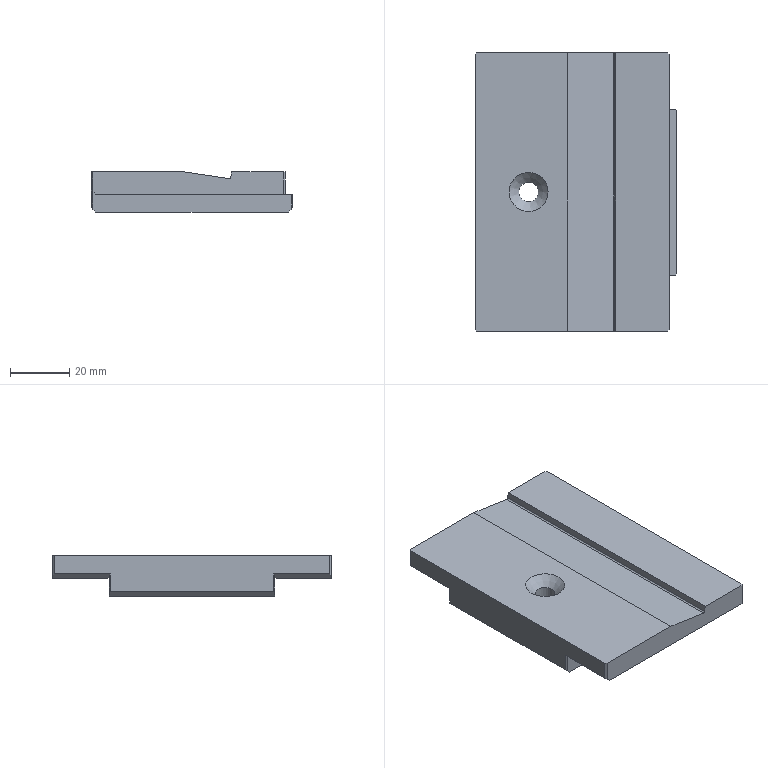NC program | NX | posted with a generic post | part box 68 x 94 x 13.65 mm
Lines 2015 to 2371 of 2371:
(FLOOR_FACING_1 , TOOL : D12精光)
N4028 T03 M6
N4030 G54
N4032 G17 G0 G90 X-44.1 Y-43.6 B0. C0. S5500 M3
N4034 G43 Z30. H3
N4036 Z-3.
N4038 G94 G1 Z-6. F800.
N4040 Y-38.6
N4042 Y37.5
N4044 X-39.1
N4046 Y-38.6
N4048 X-34.1
N4050 Y37.5
N4052 Y43.098
N4054 Z-3.
N4056 G0 Z30.
N4058 X25.1 Y43.6
N4060 Z3.
N4062 G1 Z0.
N4064 Y38.6
N4066 Y-38.6
N4068 X17.033
N4070 Y38.6
N4072 X8.967
N4074 Y-38.6
N4076 X0.9
N4078 Y38.6
N4080 X-7.167
N4082 Y-38.6
N4084 X-15.233
N4086 Y38.6
N4088 X-23.3
N4090 Y-38.6
N4092 Y-43.6
N4094 Z3.
N4096 G0 Z30.
N4098 X44.1 Y42.5
N4100 Z-3.
N4102 G1 Z-6.
N4104 Y37.5
N4106 Y-38.6
N4108 X39.1
N4110 Y37.5
N4112 X34.1
N4114 Y-38.6
N4116 Y-43.6
N4118 Z-3.
N4120 G0 Z30.
(FLOOR_FACING_1_COPY , TOOL : D12精光)
N4122 X-34. Y-40.228
N4124 Z-4.
N4126 G1 Z-6.
N4128 Y-29.5
N4130 Y28.4
N4132 Y40.228
N4134 Z-4.
N4136 G0 Z30.
N4138 X34.
N4140 Z-4.
N4142 G1 Z-6.
N4144 Y28.4
N4146 Y-29.5
N4148 Y-40.228
N4150 Z-4.
N4152 G0 Z30.
N4154 M5
(PLANAR_MILL_3 , TOOL : D4倒角刀)
N4156 T04 M6
N4158 G54
N4160 G17 G0 G90 X-29.3 Y-36. B0. C0. S4500 M3
N4162 G43 Z30. H4
N4164 Z0.5
N4166 G94 G1 Z-1.5 F1000.
N4168 Y-32.5
N4170 Y32.5
N4172 Y36.
N4174 Z0.5
N4176 G0 Z30.
N4178 X29.3
N4180 Z0.5
N4182 G1 Z-1.5
N4184 Y32.5
N4186 Y-32.5
N4188 Y-36.
N4190 Z0.5
N4192 G0 Z30.
(PLANAR_MILL_3_COPY_1 , TOOL : D4倒角刀)
N4194 X-1. Y-16.
N4196 Z0.5
N4198 G1 Z-1.5 F300.
N4200 Y-17.
N4202 G3 X0. Y-18. R1.
N4204 X2. Y-16. R2.
N4206 X0. Y-18. R-2.
N4208 X1. Y-17. R1.
N4210 G1 Y-16.
N4212 Z0.5
N4214 G0 Z30.
(PLANAR_MILL_3_COPY , TOOL : D4倒角刀)
N4216 X32. Y-34.5
N4218 Z0.2
N4220 G1 Z-1.8 F1000.
N4222 X28.
N4224 X-28.
N4226 X-32.
N4228 Z0.2
N4230 G0 Z30.
N4232 X32. Y-34.3
N4234 Z0.2
N4236 G1 Z-1.8
N4238 X28.
N4240 X-28.
N4242 X-32.
N4244 Z0.2
N4246 G0 Z30.
N4248 Y34.5
N4250 Z0.2
N4252 G1 Z-1.8
N4254 X-28.
N4256 X28.
N4258 X32.
N4260 Z0.2
N4262 G0 Z30.
N4264 X-32. Y34.3
N4266 Z0.2
N4268 G1 Z-1.8
N4270 X-28.
N4272 X28.
N4274 X32.
N4276 Z0.2
N4278 G0 Z30.
(PLANAR_MILL_3_COPY_COPY , TOOL : D4倒角刀)
N4280 X-49.5 Y-33.5
N4282 Z-5.5
N4284 G1 Z-7.5
N4286 G3 X-48.5 Y-32.5 R1.
N4288 G1 Y30.9
N4290 G2 X-48.061 Y31.961 R1.5
N4292 G1 X-47.561 Y32.461
N4294 G2 X-46.5 Y32.9 R1.5
N4296 G1 X-31.5
N4298 G3 X-30.5 Y33.9 R1.
N4300 G1 Z-5.5
N4302 G0 Z30.
N4304 X30.5
N4306 Z-5.5
N4308 G1 Z-7.5
N4310 G3 X31.5 Y32.9 R1.
N4312 G1 X46.5
N4314 G2 X47.561 Y32.461 R1.5
N4316 G1 X48.061 Y31.961
N4318 G2 X48.5 Y30.9 R1.5
N4320 G1 Y-32.5
N4322 G3 X49.5 Y-33.5 R1.
N4324 G1 Z-5.5
N4326 G0 Z30.
N4328 M5
(等高爬角 , TOOL : D4R0.5)
N4330 T07 M6
N4332 G54
N4334 G17 G0 G90 X-30.785 Y-36.372 B0. C0. S6000 M3
N4336 G43 Z30. H7
N4338 Z-5.165
N4340 G94 G1 Z-6.165 F2700.
N4342 X-29.8 Y-34.372
N4344 X-47. F3000.
N4346 Y-34.408 Z-6.201
N4348 X-29.782
N4350 X-29.764 Y-34.443 Z-6.236
N4352 X-47.
N4354 Y-34.478 Z-6.271
N4356 X-29.744
N4358 X-29.724 Y-34.514 Z-6.307
N4360 X-47.
N4362 Y-34.549 Z-6.342
N4364 X-29.703
N4366 X-29.68 Y-34.584 Z-6.377
N4368 X-47.
N4370 Y-34.62 Z-6.413
N4372 X-29.657
N4374 X-29.633 Y-34.655 Z-6.448
N4376 X-47.
N4378 Y-34.691 Z-6.483
N4380 X-29.607
N4382 X-29.58 Y-34.726 Z-6.519
N4384 X-47.
N4386 Y-34.761 Z-6.554
N4388 X-29.552
N4390 X-29.523 Y-34.797 Z-6.589
N4392 X-47.
N4394 Y-34.832 Z-6.625
N4396 X-29.492
N4398 X-29.46 Y-34.867 Z-6.66
N4400 X-47.
N4402 Y-34.903 Z-6.696
N4404 X-29.426
N4406 X-29.39 Y-34.938 Z-6.731
N4408 X-47.
N4410 Y-34.973 Z-6.766
N4412 X-29.355
N4414 X-29.32 Y-35.009 Z-6.802
N4416 X-47.
N4418 Y-35.044 Z-6.837
N4420 X-29.284
N4422 X-29.249 Y-35.079 Z-6.872
N4424 X-47.
N4426 Y-35.115 Z-6.908
N4428 X-29.214
N4430 X-29.178 Y-35.15 Z-6.943
N4432 X-47.
N4434 Y-35.185 Z-6.978
N4436 X-29.143
N4438 X-29.108 Y-35.221 Z-7.014
N4440 X-47.
N4442 Y-35.256 Z-7.049
N4444 X-29.072
N4446 X-29.037 Y-35.292 Z-7.084
N4448 X-47.
N4450 Y-35.327 Z-7.12
N4452 X-29.002
N4454 X-28.966 Y-35.362 Z-7.155
N4456 X-46.991
N4458 X-46.956 Y-35.398 Z-7.191
N4460 X-28.931
N4462 X-28.895 Y-35.433 Z-7.226
N4464 X-46.921
N4466 X-46.885 Y-35.468 Z-7.261
N4468 X-28.858
N4470 X-28.819 Y-35.504 Z-7.297
N4472 X-46.85
N4474 X-46.815 Y-35.539 Z-7.332
N4476 X-28.777
N4478 X-28.733 Y-35.574 Z-7.367
N4480 X-46.779
N4482 X-46.744 Y-35.61 Z-7.403
N4484 X-28.687
N4486 X-28.637 Y-35.645 Z-7.438
N4488 X-46.708
N4490 X-46.673 Y-35.68 Z-7.473
N4492 X-28.584
N4494 X-28.528 Y-35.716 Z-7.509
N4496 X-46.638
N4498 X-46.602 Y-35.751 Z-7.544
N4500 X-28.466
N4502 X-28.399 Y-35.787 Z-7.579
N4504 X-46.567
N4506 X-46.532 Y-35.822 Z-7.615
N4508 X-28.325
N4510 X-28.68 Y-37.822
N4512 Z-6.615
N4514 G0 Z30.
N4516 X50.387 Y-34.372
N4518 Z-5.165
N4520 G1 Z-6.165 F2700.
N4522 X47.
N4524 X29.8 F3000.
N4526 X29.782 Y-34.408 Z-6.201
N4528 X47.
N4530 Y-34.443 Z-6.236
N4532 X29.764
N4534 X29.744 Y-34.478 Z-6.271
N4536 X47.
N4538 Y-34.514 Z-6.307
N4540 X29.724
N4542 X29.703 Y-34.549 Z-6.342
N4544 X47.
N4546 Y-34.584 Z-6.377
N4548 X29.68
N4550 X29.657 Y-34.62 Z-6.413
N4552 X47.
N4554 Y-34.655 Z-6.448
N4556 X29.633
N4558 X29.607 Y-34.691 Z-6.483
N4560 X47.
N4562 Y-34.726 Z-6.519
N4564 X29.58
N4566 X29.552 Y-34.761 Z-6.554
N4568 X47.
N4570 Y-34.797 Z-6.589
N4572 X29.523
N4574 X29.492 Y-34.832 Z-6.625
N4576 X47.
N4578 Y-34.867 Z-6.66
N4580 X29.46
N4582 X29.426 Y-34.903 Z-6.696
N4584 X47.
N4586 Y-34.938 Z-6.731
N4588 X29.39
N4590 X29.355 Y-34.973 Z-6.766
N4592 X47.
N4594 Y-35.009 Z-6.802
N4596 X29.32
N4598 X29.284 Y-35.044 Z-6.837
N4600 X47.
N4602 Y-35.079 Z-6.872
N4604 X29.249
N4606 X29.214 Y-35.115 Z-6.908
N4608 X47.
N4610 Y-35.15 Z-6.943
N4612 X29.178
N4614 X29.143 Y-35.185 Z-6.978
N4616 X47.
N4618 Y-35.221 Z-7.014
N4620 X29.108
N4622 X29.072 Y-35.256 Z-7.049
N4624 X47.
N4626 Y-35.292 Z-7.084
N4628 X29.037
N4630 X29.002 Y-35.327 Z-7.12
N4632 X47.
N4634 X46.991 Y-35.362 Z-7.155
N4636 X28.966
N4638 X28.931 Y-35.398 Z-7.191
N4640 X46.956
N4642 X46.921 Y-35.433 Z-7.226
N4644 X28.895
N4646 X28.858 Y-35.468 Z-7.261
N4648 X46.885
N4650 X46.85 Y-35.504 Z-7.297
N4652 X28.819
N4654 X28.777 Y-35.539 Z-7.332
N4656 X46.815
N4658 X46.779 Y-35.574 Z-7.367
N4660 X28.733
N4662 X28.687 Y-35.61 Z-7.403
N4664 X46.744
N4666 X46.708 Y-35.645 Z-7.438
N4668 X28.637
N4670 X28.584 Y-35.68 Z-7.473
N4672 X46.673
N4674 X46.638 Y-35.716 Z-7.509
N4676 X28.528
N4678 X28.466 Y-35.751 Z-7.544
N4680 X46.602
N4682 X46.567 Y-35.787 Z-7.579
N4684 X28.399
N4686 X28.325 Y-35.822 Z-7.615
N4688 X46.532
N4690 X50.257
N4692 Z-6.615
N4694 G0 Z30.
N4696 M5
N4698 M2